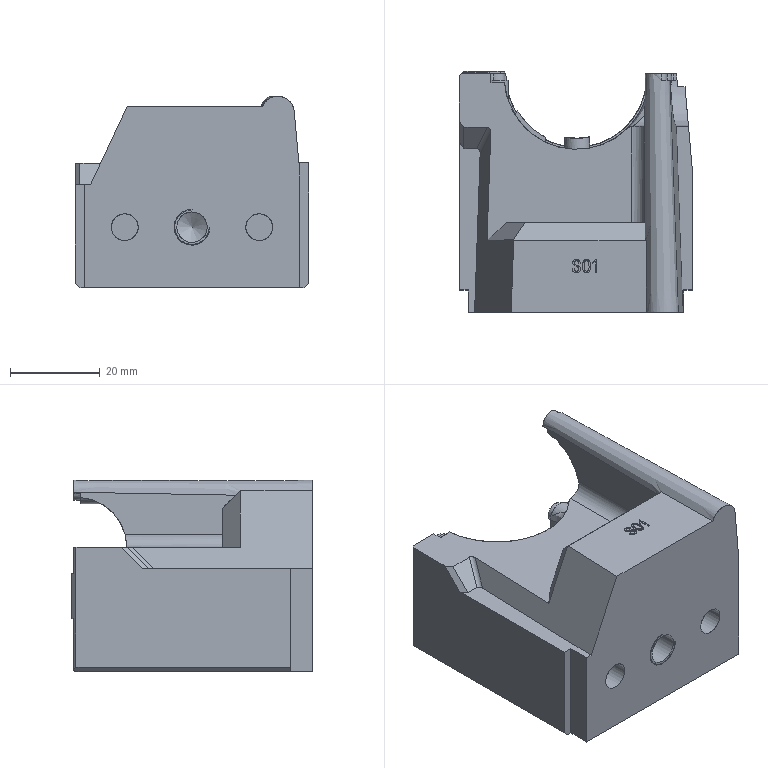NC program | PowerMill | posted with a generic post | part box 52 x 53.756 x 42.711 mm
Whole program:
%
O0001
N104 ( POWERMILL CB  : 2026004.0)
N105 ( POST VER      : 2026.0.0.5161)
N106 ( OPTION FILE   : FANUC)
N107 ( OUTPUT WORKPLANE : 1)
N108 (  )
N109 ( TOOL LIST )
N110 (--------------------------------)
N111 ( NO. | ID | DIA.| TIP RAD|LENGTH)
N112 (--------------------------------)
N113 (    1|D8_1| 8.0 |  0.0   | 99.0 )
N114 (--------------------------------)
N115 (  )
N116 ( NUMBER OF TOOLPATHS: 1.0 )
N117 ( ESTIMATED PROGRAM DURATION: 0 HOURS 1 MIN 2 SEC)
N118 (  )
N119 G00 G21 G80 G40 G17
N120 G90
N121 G54
N122 G53 Z0.0
N123 (---------------)
N124 ( START TOOLPATH : 01开粗-D8-等高 )
N125 (---------------)
N126 ( TOOL NO.    :1 )
N127 ( TOOL TYPE   : ENDMILL)
N128 ( TOOL ID     : D8_1)
N129 ( TOOL DIA    : 8.0 LENGTH 99.0)
N130 T1
N131 M6
N132 S3500 M03
N133 G00 G90 X28.4144 Y-5.6
N134 G43 Z20.0 H1
N135
N136 G05 P10000 R8
N137 Z2.8528
N138 G01 Z-0.1472 F2100.0
N139 G02 X28.2 Y-4.8 I1.3856 J0.8 F3500.0
N140 G01 Y0.0
N141 Y42.71
N142 Y47.51
N143 G02 X28.4144 Y48.31 I1.6 J0.0
N144 G01 X28.4404 Y48.3551 Z-0.1688
N145 X28.4512 Y48.3738 Z-0.2209
N146 X28.4404 Y48.3551 Z-0.2729
N147 X28.4144 Y48.31 Z-0.2945
N148 G03 X28.2 Y47.51 I1.3856 J-0.8
N149 G01 Y42.71
N150 Y0.0
N151 Y-4.8
N152 G03 X28.4144 Y-5.6 I1.6 J0.0
N153 G01 X28.4404 Y-5.6451 Z-0.316
N154 X28.4512 Y-5.6638 Z-0.3681
N155 X28.4404 Y-5.6451 Z-0.4201
N156 X28.4144 Y-5.6 Z-0.4417
N157 G02 X28.2 Y-4.8 I1.3856 J0.8
N158 G01 Y0.0
N159 Y42.71
N160 Y47.51
N161 G02 X28.4144 Y48.31 I1.6 J0.0
N162 G01 X28.4404 Y48.3551 Z-0.4633
N163 X28.4512 Y48.3738 Z-0.5153
N164 X28.4404 Y48.3551 Z-0.5674
N165 X28.4144 Y48.31 Z-0.5889
N166 G03 X28.2 Y47.51 I1.3856 J-0.8
N167 G01 Y42.71
N168 Y0.0
N169 Y-4.8
N170 G03 X28.4144 Y-5.6 I1.6 J0.0
N171 G01 X28.4404 Y-5.6451 Z-0.6105
N172 X28.4512 Y-5.6638 Z-0.6626
N173 X28.4404 Y-5.6451 Z-0.7146
N174 X28.4144 Y-5.6 Z-0.7362
N175 G02 X28.2 Y-4.8 I1.3856 J0.8
N176 G01 Y0.0
N177 Y42.71
N178 Y47.51
N179 G02 X28.4144 Y48.31 I1.6 J0.0
N180 G01 X28.4404 Y48.3551 Z-0.7577
N181 X28.4512 Y48.3738 Z-0.8098
N182 X28.4404 Y48.3551 Z-0.8618
N183 X28.4144 Y48.31 Z-0.8834
N184 G03 X28.2 Y47.51 I1.3856 J-0.8
N185 G01 Y42.71
N186 Y0.0
N187 Y-4.8
N188 G03 X28.4144 Y-5.6 I1.6 J0.0
N189 G01 X28.4404 Y-5.6451 Z-0.905
N190 X28.4512 Y-5.6638 Z-0.957
N191 X28.4404 Y-5.6451 Z-1.0091
N192 X28.4144 Y-5.6 Z-1.0306
N193 G02 X28.2 Y-4.8 I1.3856 J0.8
N194 G01 Y0.0
N195 Y42.71
N196 Y47.51
N197 G02 X28.4144 Y48.31 I1.6 J0.0
N198 G01 X28.4404 Y48.3551 Z-1.0522
N199 X28.4512 Y48.3738 Z-1.1043
N200 X28.4404 Y48.3551 Z-1.1563
N201 X28.4144 Y48.31 Z-1.1779
N202 G03 X28.2 Y47.51 I1.3856 J-0.8
N203 G01 Y42.71
N204 Y0.0
N205 Y-4.8
N206 G03 X28.4144 Y-5.6 I1.6 J0.0
N207 G01 X28.4404 Y-5.6451 Z-1.1994
N208 X28.4512 Y-5.6638 Z-1.2515
N209 X28.4404 Y-5.6451 Z-1.3036
N210 X28.4144 Y-5.6 Z-1.3251
N211 G02 X28.2 Y-4.8 I1.3856 J0.8
N212 G01 Y0.0
N213 Y42.71
N214 Y47.51
N215 G02 X28.4144 Y48.31 I1.6 J0.0
N216 G01 X28.4404 Y48.3551 Z-1.3467
N217 X28.4512 Y48.3738 Z-1.3987
N218 X28.4404 Y48.3551 Z-1.4508
N219 X28.4144 Y48.31 Z-1.4724
N220 G03 X28.2 Y47.51 I1.3856 J-0.8
N221 G01 Y42.71
N222 Y0.0
N223 Y-4.8
N224 G03 X28.4144 Y-5.6 I1.6 J0.0
N225 G01 X28.4404 Y-5.6451 Z-1.4939
N226 X28.4512 Y-5.6638 Z-1.546
N227 X28.4404 Y-5.6451 Z-1.598
N228 X28.4144 Y-5.6 Z-1.6196
N229 G02 X28.2 Y-4.8 I1.3856 J0.8
N230 G01 Y0.0
N231 Y42.71
N232 Y47.51
N233 G02 X28.4144 Y48.31 I1.6 J0.0
N234 G01 X28.4404 Y48.3551 Z-1.6412
N235 X28.4512 Y48.3738 Z-1.6932
N236 X28.4404 Y48.3551 Z-1.7453
N237 X28.4144 Y48.31 Z-1.7668
N238 G03 X28.2 Y47.51 I1.3856 J-0.8
N239 G01 Y42.71
N240 Y0.0
N241 Y-4.8
N242 G03 X28.4144 Y-5.6 I1.6 J0.0
N243 G01 X28.4404 Y-5.6451 Z-1.7884
N244 X28.4512 Y-5.6638 Z-1.8404
N245 X28.4404 Y-5.6451 Z-1.8925
N246 X28.4144 Y-5.6 Z-1.9141
N247 G02 X28.2 Y-4.8 I1.3856 J0.8
N248 G01 Y0.0
N249 Y42.71
N250 Y47.51
N251 G02 X28.4144 Y48.31 I1.6 J0.0
N252 G01 X28.4404 Y48.3551 Z-1.9356
N253 X28.4512 Y48.3738 Z-1.9877
N254 X28.4404 Y48.3551 Z-2.0397
N255 X28.4144 Y48.31 Z-2.0613
N256 G03 X28.2 Y47.51 I1.3856 J-0.8
N257 G01 Y42.71
N258 Y0.0
N259 Y-4.8
N260 G03 X28.4144 Y-5.6 I1.6 J0.0
N261 G01 X28.4404 Y-5.6451 Z-2.0829
N262 X28.4512 Y-5.6638 Z-2.1349
N263 X28.4404 Y-5.6451 Z-2.187
N264 X28.4144 Y-5.6 Z-2.2085
N265 G02 X28.2 Y-4.8 I1.3856 J0.8
N266 G01 Y0.0
N267 Y42.71
N268 Y47.51
N269 G02 X28.4144 Y48.31 I1.6 J0.0
N270 G01 X28.4404 Y48.3551 Z-2.2301
N271 X28.4512 Y48.3738 Z-2.2821
N272 X28.4404 Y48.3551 Z-2.3342
N273 X28.4144 Y48.31 Z-2.3558
N274 G03 X28.2 Y47.51 I1.3856 J-0.8
N275 G01 Y42.71
N276 Y0.0
N277 Y-4.8
N278 G03 X28.4144 Y-5.6 I1.6 J0.0
N279 G01 X28.4404 Y-5.6451 Z-2.3773
N280 X28.4512 Y-5.6638 Z-2.4294
N281 X28.4404 Y-5.6451 Z-2.4814
N282 X28.4144 Y-5.6 Z-2.503
N283 G02 X28.2 Y-4.8 I1.3856 J0.8
N284 G01 Y0.0
N285 Y42.71
N286 Y47.51
N287 G02 X28.4144 Y48.31 I1.6 J0.0
N288 G01 X28.4404 Y48.3551 Z-2.5246
N289 X28.4512 Y48.3738 Z-2.5766
N290 X28.4404 Y48.3551 Z-2.6287
N291 X28.4144 Y48.31 Z-2.6502
N292 G03 X28.2 Y47.51 I1.3856 J-0.8
N293 G01 Y42.71
N294 Y0.0
N295 Y-4.8
N296 G03 X28.4144 Y-5.6 I1.6 J0.0
N297 G01 X28.4404 Y-5.6451 Z-2.6718
N298 X28.4512 Y-5.6638 Z-2.7239
N299 X28.4404 Y-5.6451 Z-2.7759
N300 X28.4144 Y-5.6 Z-2.7975
N301 G02 X28.2 Y-4.8 I1.3856 J0.8
N302 G01 Y0.0
N303 Y42.71
N304 Y47.51
N305 G02 X28.4144 Y48.31 I1.6 J0.0
N306 G01 X28.4404 Y48.3551 Z-2.819
N307 X28.4512 Y48.3738 Z-2.8711
N308 X28.4404 Y48.3551 Z-2.9231
N309 X28.4144 Y48.31 Z-2.9447
N310 G03 X28.2 Y47.51 I1.3856 J-0.8
N311 G01 Y42.71
N312 Y0.0
N313 Y-4.8
N314 G03 X28.4144 Y-5.6 I1.6 J0.0
N315 G01 X28.4404 Y-5.6451 Z-2.9663
N316 X28.4512 Y-5.6638 Z-3.0183
N317 X28.4404 Y-5.6451 Z-3.0704
N318 X28.4144 Y-5.6 Z-3.0919
N319 G02 X28.2 Y-4.8 I1.3856 J0.8
N320 G01 Y0.0
N321 Y42.71
N322 Y47.51
N323 G02 X28.4144 Y48.31 I1.6 J0.0
N324 G01 X28.4404 Y48.3551 Z-3.1135
N325 X28.4512 Y48.3738 Z-3.1656
N326 X28.4404 Y48.3551 Z-3.2176
N327 X28.4144 Y48.31 Z-3.2392
N328 G03 X28.2 Y47.51 I1.3856 J-0.8
N329 G01 Y42.71
N330 Y0.0
N331 Y-4.8
N332 G03 X28.4144 Y-5.6 I1.6 J0.0
N333 G01 X28.4404 Y-5.6451 Z-3.2607
N334 X28.4512 Y-5.6638 Z-3.3128
N335 X28.4404 Y-5.6451 Z-3.3648
N336 X28.4144 Y-5.6 Z-3.3864
N337 G02 X28.2 Y-4.8 I1.3856 J0.8
N338 G01 Y0.0
N339 Y42.71
N340 Y47.51
N341 G02 X28.4144 Y48.31 I1.6 J0.0
N342 G01 X28.4404 Y48.3551 Z-3.408
N343 X28.4512 Y48.3738 Z-3.46
N344 X28.4404 Y48.3551 Z-3.5121
N345 X28.4144 Y48.31 Z-3.5336
N346 G03 X28.2 Y47.51 I1.3856 J-0.8
N347 G01 Y42.71
N348 Y0.0
N349 Y-4.8
N350 G03 X28.4144 Y-5.6 I1.6 J0.0
N351 G01 X28.4404 Y-5.6451 Z-3.5552
N352 X28.4512 Y-5.6638 Z-3.6073
N353 X28.4404 Y-5.6451 Z-3.6593
N354 X28.4144 Y-5.6 Z-3.6809
N355 G02 X28.2 Y-4.8 I1.3856 J0.8
N356 G01 Y0.0
N357 Y42.71
N358 Y47.51
N359 G02 X28.4144 Y48.31 I1.6 J0.0
N360 G01 X28.4404 Y48.3551 Z-3.7024
N361 X28.4512 Y48.3738 Z-3.7545
N362 X28.4404 Y48.3551 Z-3.8066
N363 X28.4144 Y48.31 Z-3.8281
N364 G03 X28.2 Y47.51 I1.3856 J-0.8
N365 G01 Y42.71
N366 Y0.0
N367 Y-4.8
N368 G03 X28.4144 Y-5.6 I1.6 J0.0
N369 G01 X28.4404 Y-5.6451 Z-3.8497
N370 X28.4512 Y-5.6638 Z-3.9017
N371 X28.4404 Y-5.6451 Z-3.9538
N372 X28.4144 Y-5.6 Z-3.9754
N373 G02 X28.2 Y-4.8 I1.3856 J0.8
N374 G01 Y0.0
N375 Y42.71
N376 Y47.51
N377 G02 X28.4144 Y48.31 I1.6 J0.0
N378 G01 X28.4404 Y48.3551 Z-3.9969
N379 X28.4512 Y48.3738 Z-4.049
N380 X28.4404 Y48.3551 Z-4.101
N381 X28.4144 Y48.31 Z-4.1226
N382 G03 X28.2 Y47.51 I1.3856 J-0.8
N383 G01 Y42.71
N384 Y0.0
N385 Y-4.8
N386 G03 X28.4144 Y-5.6 I1.6 J0.0
N387 G01 X28.4404 Y-5.6451 Z-4.1442
N388 X28.4512 Y-5.6638 Z-4.1962
N389 X28.4404 Y-5.6451 Z-4.2483
N390 X28.4144 Y-5.6 Z-4.2698
N391 G02 X28.2 Y-4.8 I1.3856 J0.8
N392 G01 Y0.0
N393 Y42.71
N394 Y47.51
N395 G02 X28.4144 Y48.31 I1.6 J0.0
N396 G01 X28.4404 Y48.3551 Z-4.2914
N397 X28.4512 Y48.3738 Z-4.3434
N398 X28.4404 Y48.3551 Z-4.3955
N399 X28.4144 Y48.31 Z-4.4171
N400 G03 X28.2 Y47.51 I1.3856 J-0.8
N401 G01 Y42.71
N402 Y0.0
N403 Y-4.8
N404 G03 X28.4144 Y-5.6 I1.6 J0.0
N405 G01 X28.4404 Y-5.6451 Z-4.4386
N406 X28.4512 Y-5.6638 Z-4.4907
N407 X28.4404 Y-5.6451 Z-4.5427
N408 X28.4144 Y-5.6 Z-4.5643
N409 G02 X28.2 Y-4.8 I1.3856 J0.8
N410 G01 Y0.0
N411 Y42.71
N412 Y47.51
N413 G02 X28.4144 Y48.31 I1.6 J0.0
N414 G01 X28.4404 Y48.3551 Z-4.5859
N415 X28.4512 Y48.3738 Z-4.6379
N416 X28.4404 Y48.3551 Z-4.69
N417 X28.4144 Y48.31 Z-4.7115
N418 G03 X28.2 Y47.51 I1.3856 J-0.8
N419 G01 Y42.71
N420 Y0.0
N421 Y-4.8
N422 G03 X28.4144 Y-5.6 I1.6 J0.0
N423 G01 X28.4404 Y-5.6451 Z-4.7331
N424 X28.4512 Y-5.6638 Z-4.7851
N425 X28.4404 Y-5.6451 Z-4.8372
N426 X28.4144 Y-5.6 Z-4.8588
N427 G02 X28.2 Y-4.8 I1.3856 J0.8
N428 G01 Y0.0
N429 Y42.71
N430 Y47.51
N431 G02 X28.4144 Y48.31 I1.6 J0.0
N432 G00 Z5.2641
N433 G01 X-28.4144 Y-5.6 F10000.0
N434 G00 Z2.8528
N435 G01 Z-0.1472 F2100.0
N436 G03 X-28.2 Y-4.8 I-1.3856 J0.8 F3500.0
N437 G01 Y0.0
N438 Y42.71
N439 Y47.51
N440 G03 X-28.4144 Y48.31 I-1.6 J0.0
N441 G01 X-28.4404 Y48.3551 Z-0.1688
N442 X-28.4512 Y48.3738 Z-0.2209
N443 X-28.4404 Y48.3551 Z-0.2729
N444 X-28.4144 Y48.31 Z-0.2945
N445 G02 X-28.2 Y47.51 I-1.3856 J-0.8
N446 G01 Y42.71
N447 Y0.0
N448 Y-4.8
N449 G02 X-28.4144 Y-5.6 I-1.6 J0.0
N450 G01 X-28.4404 Y-5.6451 Z-0.316
N451 X-28.4512 Y-5.6638 Z-0.3681
N452 X-28.4404 Y-5.6451 Z-0.4201
N453 X-28.4144 Y-5.6 Z-0.4417
N454 G03 X-28.2 Y-4.8 I-1.3856 J0.8
N455 G01 Y0.0
N456 Y42.71
N457 Y47.51
N458 G03 X-28.4144 Y48.31 I-1.6 J0.0
N459 G01 X-28.4404 Y48.3551 Z-0.4633
N460 X-28.4512 Y48.3738 Z-0.5153
N461 X-28.4404 Y48.3551 Z-0.5674
N462 X-28.4144 Y48.31 Z-0.5889
N463 G02 X-28.2 Y47.51 I-1.3856 J-0.8
N464 G01 Y42.71
N465 Y0.0
N466 Y-4.8
N467 G02 X-28.4144 Y-5.6 I-1.6 J0.0
N468 G01 X-28.4404 Y-5.6451 Z-0.6105
N469 X-28.4512 Y-5.6638 Z-0.6626
N470 X-28.4404 Y-5.6451 Z-0.7146
N471 X-28.4144 Y-5.6 Z-0.7362
N472 G03 X-28.2 Y-4.8 I-1.3856 J0.8
N473 G01 Y0.0
N474 Y42.71
N475 Y47.51
N476 G03 X-28.4144 Y48.31 I-1.6 J0.0
N477 G01 X-28.4404 Y48.3551 Z-0.7577
N478 X-28.4512 Y48.3738 Z-0.8098
N479 X-28.4404 Y48.3551 Z-0.8618
N480 X-28.4144 Y48.31 Z-0.8834
N481 G02 X-28.2 Y47.51 I-1.3856 J-0.8
N482 G01 Y42.71
N483 Y0.0
N484 Y-4.8
N485 G02 X-28.4144 Y-5.6 I-1.6 J0.0
N486 G01 X-28.4404 Y-5.6451 Z-0.905
N487 X-28.4512 Y-5.6638 Z-0.957
N488 X-28.4404 Y-5.6451 Z-1.0091
N489 X-28.4144 Y-5.6 Z-1.0306
N490 G03 X-28.2 Y-4.8 I-1.3856 J0.8
N491 G01 Y0.0
N492 Y42.71
N493 Y47.51
N494 G03 X-28.4144 Y48.31 I-1.6 J0.0
N495 G01 X-28.4404 Y48.3551 Z-1.0522
N496 X-28.4512 Y48.3738 Z-1.1043
N497 X-28.4404 Y48.3551 Z-1.1563
N498 X-28.4144 Y48.31 Z-1.1779
N499 G02 X-28.2 Y47.51 I-1.3856 J-0.8
N500 G01 Y42.71
N501 Y0.0
N502 Y-4.8
N503 G02 X-28.4144 Y-5.6 I-1.6 J0.0
N504 G01 X-28.4404 Y-5.6451 Z-1.1994
N505 X-28.4512 Y-5.6638 Z-1.2515
N506 X-28.4404 Y-5.6451 Z-1.3036
N507 X-28.4144 Y-5.6 Z-1.3251
N508 G03 X-28.2 Y-4.8 I-1.3856 J0.8
N509 G01 Y0.0
N510 Y42.71
N511 Y47.51
N512 G03 X-28.4144 Y48.31 I-1.6 J0.0
N513 G01 X-28.4404 Y48.3551 Z-1.3467
N514 X-28.4512 Y48.3738 Z-1.3987
N515 X-28.4404 Y48.3551 Z-1.4508
N516 X-28.4144 Y48.31 Z-1.4724
N517 G02 X-28.2 Y47.51 I-1.3856 J-0.8
N518 G01 Y42.71
N519 Y0.0
N520 Y-4.8
N521 G02 X-28.4144 Y-5.6 I-1.6 J0.0
N522 G01 X-28.4404 Y-5.6451 Z-1.4939
N523 X-28.4512 Y-5.6638 Z-1.546
N524 X-28.4404 Y-5.6451 Z-1.598
N525 X-28.4144 Y-5.6 Z-1.6196
N526 G03 X-28.2 Y-4.8 I-1.3856 J0.8
N527 G01 Y0.0
N528 Y42.71
N529 Y47.51
N530 G03 X-28.4144 Y48.31 I-1.6 J0.0
N531 G01 X-28.4404 Y48.3551 Z-1.6412
N532 X-28.4512 Y48.3738 Z-1.6932
N533 X-28.4404 Y48.3551 Z-1.7453
N534 X-28.4144 Y48.31 Z-1.7668
N535 G02 X-28.2 Y47.51 I-1.3856 J-0.8
N536 G01 Y42.71
N537 Y0.0
N538 Y-4.8
N539 G02 X-28.4144 Y-5.6 I-1.6 J0.0
N540 G01 X-28.4404 Y-5.6451 Z-1.7884
N541 X-28.4512 Y-5.6638 Z-1.8404
N542 X-28.4404 Y-5.6451 Z-1.8925
N543 X-28.4144 Y-5.6 Z-1.9141
N544 G03 X-28.2 Y-4.8 I-1.3856 J0.8
N545 G01 Y0.0
N546 Y42.71
N547 Y47.51
N548 G03 X-28.4144 Y48.31 I-1.6 J0.0
N549 G01 X-28.4404 Y48.3551 Z-1.9356
N550 X-28.4512 Y48.3738 Z-1.9877
N551 X-28.4404 Y48.3551 Z-2.0397
N552 X-28.4144 Y48.31 Z-2.0613
N553 G02 X-28.2 Y47.51 I-1.3856 J-0.8
N554 G01 Y42.71
N555 Y0.0
N556 Y-4.8
N557 G02 X-28.4144 Y-5.6 I-1.6 J0.0
N558 G01 X-28.4404 Y-5.6451 Z-2.0829
N559 X-28.4512 Y-5.6638 Z-2.1349
N560 X-28.4404 Y-5.6451 Z-2.187
N561 X-28.4144 Y-5.6 Z-2.2085
N562 G03 X-28.2 Y-4.8 I-1.3856 J0.8
N563 G01 Y0.0
N564 Y42.71
N565 Y47.51
N566 G03 X-28.4144 Y48.31 I-1.6 J0.0
N567 G01 X-28.4404 Y48.3551 Z-2.2301
N568 X-28.4512 Y48.3738 Z-2.2821
N569 X-28.4404 Y48.3551 Z-2.3342
N570 X-28.4144 Y48.31 Z-2.3558
N571 G02 X-28.2 Y47.51 I-1.3856 J-0.8
N572 G01 Y42.71
N573 Y0.0
N574 Y-4.8
N575 G02 X-28.4144 Y-5.6 I-1.6 J0.0
N576 G01 X-28.4404 Y-5.6451 Z-2.3773
N577 X-28.4512 Y-5.6638 Z-2.4294
N578 X-28.4404 Y-5.6451 Z-2.4814
N579 X-28.4144 Y-5.6 Z-2.503
N580 G03 X-28.2 Y-4.8 I-1.3856 J0.8
N581 G01 Y0.0
N582 Y42.71
N583 Y47.51
N584 G03 X-28.4144 Y48.31 I-1.6 J0.0
N585 G01 X-28.4404 Y48.3551 Z-2.5246
N586 X-28.4512 Y48.3738 Z-2.5766
N587 X-28.4404 Y48.3551 Z-2.6287
N588 X-28.4144 Y48.31 Z-2.6502
N589 G02 X-28.2 Y47.51 I-1.3856 J-0.8
N590 G01 Y42.71
N591 Y0.0
N592 Y-4.8
N593 G02 X-28.4144 Y-5.6 I-1.6 J0.0
N594 G01 X-28.4404 Y-5.6451 Z-2.6718
N595 X-28.4512 Y-5.6638 Z-2.7239
N596 X-28.4404 Y-5.6451 Z-2.7759
N597 X-28.4144 Y-5.6 Z-2.7975
N598 G03 X-28.2 Y-4.8 I-1.3856 J0.8
N599 G01 Y0.0
N600 Y42.71
N601 Y47.51
N602 G03 X-28.4144 Y48.31 I-1.6 J0.0
N603 G01 X-28.4404 Y48.3551 Z-2.819
N604 X-28.4512 Y48.3738 Z-2.8711
N605 X-28.4404 Y48.3551 Z-2.9231
N606 X-28.4144 Y48.31 Z-2.9447
N607 G02 X-28.2 Y47.51 I-1.3856 J-0.8
N608 G01 Y42.71
N609 Y0.0
N610 Y-4.8
N611 G02 X-28.4144 Y-5.6 I-1.6 J0.0
N612 G01 X-28.4404 Y-5.6451 Z-2.9663
N613 X-28.4512 Y-5.6638 Z-3.0183
N614 X-28.4404 Y-5.6451 Z-3.0704
N615 X-28.4144 Y-5.6 Z-3.0919
N616 G03 X-28.2 Y-4.8 I-1.3856 J0.8
N617 G01 Y0.0
N618 Y42.71
N619 Y47.51
N620 G03 X-28.4144 Y48.31 I-1.6 J0.0
N621 G01 X-28.4404 Y48.3551 Z-3.1135
N622 X-28.4512 Y48.3738 Z-3.1656
N623 X-28.4404 Y48.3551 Z-3.2176
N624 X-28.4144 Y48.31 Z-3.2392
N625 G02 X-28.2 Y47.51 I-1.3856 J-0.8
N626 G01 Y42.71
N627 Y0.0
N628 Y-4.8
N629 G02 X-28.4144 Y-5.6 I-1.6 J0.0
N630 G01 X-28.4404 Y-5.6451 Z-3.2607
N631 X-28.4512 Y-5.6638 Z-3.3128
N632 X-28.4404 Y-5.6451 Z-3.3648
N633 X-28.4144 Y-5.6 Z-3.3864
N634 G03 X-28.2 Y-4.8 I-1.3856 J0.8
N635 G01 Y0.0
N636 Y42.71
N637 Y47.51
N638 G03 X-28.4144 Y48.31 I-1.6 J0.0
N639 G01 X-28.4404 Y48.3551 Z-3.408
N640 X-28.4512 Y48.3738 Z-3.46
N641 X-28.4404 Y48.3551 Z-3.5121
N642 X-28.4144 Y48.31 Z-3.5336
N643 G02 X-28.2 Y47.51 I-1.3856 J-0.8
N644 G01 Y42.71
N645 Y0.0
N646 Y-4.8
N647 G02 X-28.4144 Y-5.6 I-1.6 J0.0
N648 G01 X-28.4404 Y-5.6451 Z-3.5552
N649 X-28.4512 Y-5.6638 Z-3.6073
N650 X-28.4404 Y-5.6451 Z-3.6593
N651 X-28.4144 Y-5.6 Z-3.6809
N652 G03 X-28.2 Y-4.8 I-1.3856 J0.8
N653 G01 Y0.0
N654 Y42.71
N655 Y47.51
N656 G03 X-28.4144 Y48.31 I-1.6 J0.0
N657 G01 X-28.4404 Y48.3551 Z-3.7024
N658 X-28.4512 Y48.3738 Z-3.7545
N659 X-28.4404 Y48.3551 Z-3.8066
N660 X-28.4144 Y48.31 Z-3.8281
N661 G02 X-28.2 Y47.51 I-1.3856 J-0.8
N662 G01 Y42.71
N663 Y0.0
N664 Y-4.8
N665 G02 X-28.4144 Y-5.6 I-1.6 J0.0
N666 G01 X-28.4404 Y-5.6451 Z-3.8497
N667 X-28.4512 Y-5.6638 Z-3.9017
N668 X-28.4404 Y-5.6451 Z-3.9538
N669 X-28.4144 Y-5.6 Z-3.9754
N670 G03 X-28.2 Y-4.8 I-1.3856 J0.8
N671 G01 Y0.0
N672 Y42.71
N673 Y47.51
N674 G03 X-28.4144 Y48.31 I-1.6 J0.0
N675 G01 X-28.4404 Y48.3551 Z-3.9969
N676 X-28.4512 Y48.3738 Z-4.049
N677 X-28.4404 Y48.3551 Z-4.101
N678 X-28.4144 Y48.31 Z-4.1226
N679 G02 X-28.2 Y47.51 I-1.3856 J-0.8
N680 G01 Y42.71
N681 Y0.0
N682 Y-4.8
N683 G02 X-28.4144 Y-5.6 I-1.6 J0.0
N684 G01 X-28.4404 Y-5.6451 Z-4.1442
N685 X-28.4512 Y-5.6638 Z-4.1962
N686 X-28.4404 Y-5.6451 Z-4.2483
N687 X-28.4144 Y-5.6 Z-4.2698
N688 G03 X-28.2 Y-4.8 I-1.3856 J0.8
N689 G01 Y0.0
N690 Y42.71
N691 Y47.51
N692 G03 X-28.4144 Y48.31 I-1.6 J0.0
N693 G01 X-28.4404 Y48.3551 Z-4.2914
N694 X-28.4512 Y48.3738 Z-4.3434
N695 X-28.4404 Y48.3551 Z-4.3955
N696 X-28.4144 Y48.31 Z-4.4171
N697 G02 X-28.2 Y47.51 I-1.3856 J-0.8
N698 G01 Y42.71
N699 Y0.0
N700 Y-4.8
N701 G02 X-28.4144 Y-5.6 I-1.6 J0.0
N702 G01 X-28.4404 Y-5.6451 Z-4.4386
N703 X-28.4512 Y-5.6638 Z-4.4907
N704 X-28.4404 Y-5.6451 Z-4.5427
N705 X-28.4144 Y-5.6 Z-4.5643
N706 G03 X-28.2 Y-4.8 I-1.3856 J0.8
N707 G01 Y0.0
N708 Y42.71
N709 Y47.51
N710 G03 X-28.4144 Y48.31 I-1.6 J0.0
N711 G01 X-28.4404 Y48.3551 Z-4.5859
N712 X-28.4512 Y48.3738 Z-4.6379
N713 X-28.4404 Y48.3551 Z-4.69
N714 X-28.4144 Y48.31 Z-4.7115
N715 G02 X-28.2 Y47.51 I-1.3856 J-0.8
N716 G01 Y42.71
N717 Y0.0
N718 Y-4.8
N719 G02 X-28.4144 Y-5.6 I-1.6 J0.0
N720 G01 X-28.4404 Y-5.6451 Z-4.7331
N721 X-28.4512 Y-5.6638 Z-4.7851
N722 X-28.4404 Y-5.6451 Z-4.8372
N723 X-28.4144 Y-5.6 Z-4.8588
N724 G03 X-28.2 Y-4.8 I-1.3856 J0.8
N725 G01 Y0.0
N726 Y42.71
N727 Y47.51
N728 G03 X-28.4144 Y48.31 I-1.6 J0.0
N729 G00 Z20.0
N730 G05 P0
N731 (---------------)
N732 ( END TOOLPATH : 01开粗-D8-等高 )
N733 (---------------)
N734
N735 M05
N736 G53 Z0.0
N737 M30
%